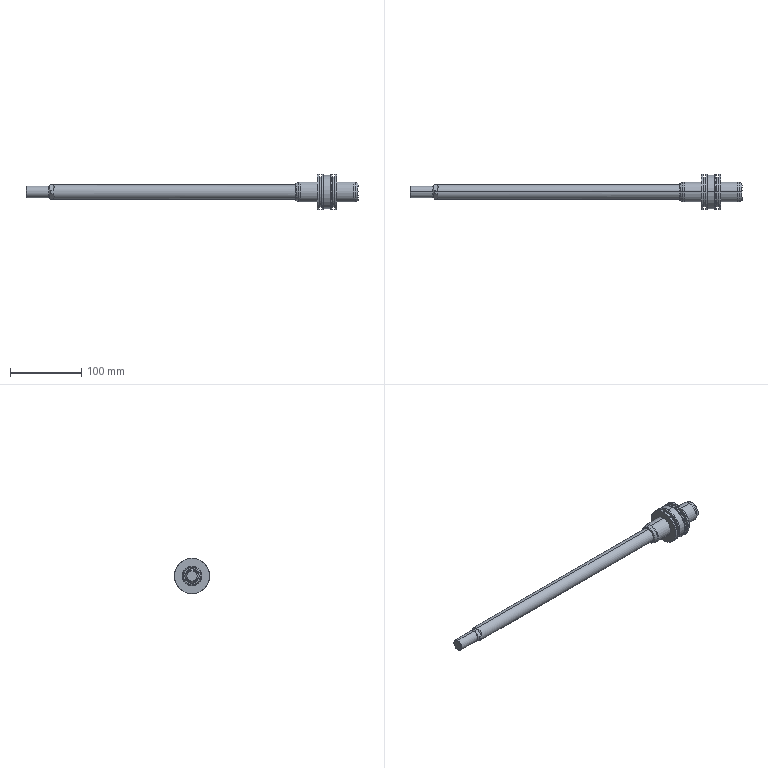Part | SolidWorks | features BaseBody 1 | 1 solid | 84 faces | box 465.5 x 49.5 x 49.5 mm | volume 181589 mm3 | cone 28 | cylinder 24 | plane 20 | spline 12 | commonest cylinder face diameters 49.5 x8 28 x4 42 x4 16 x2 19 x2 20 x2